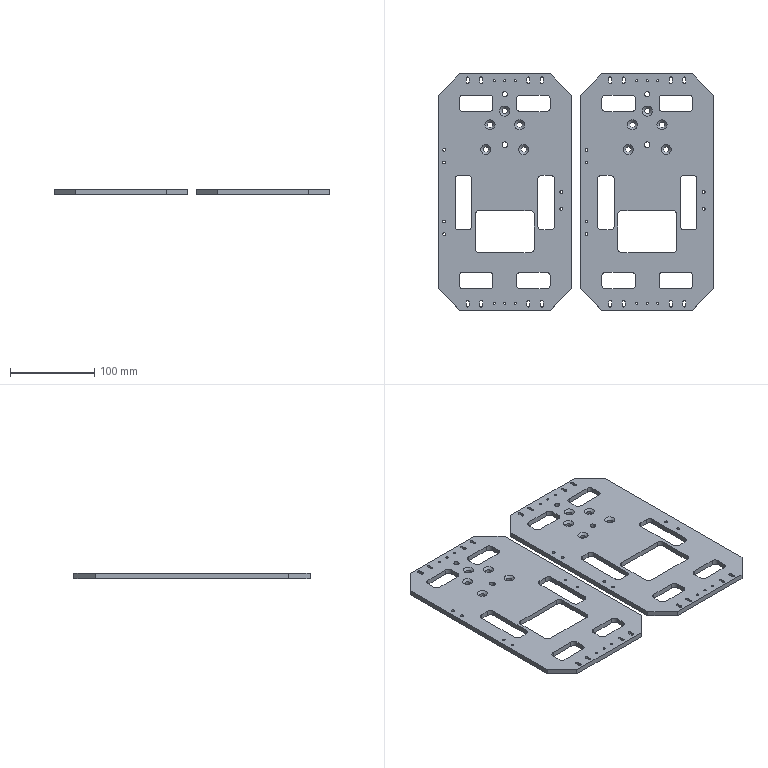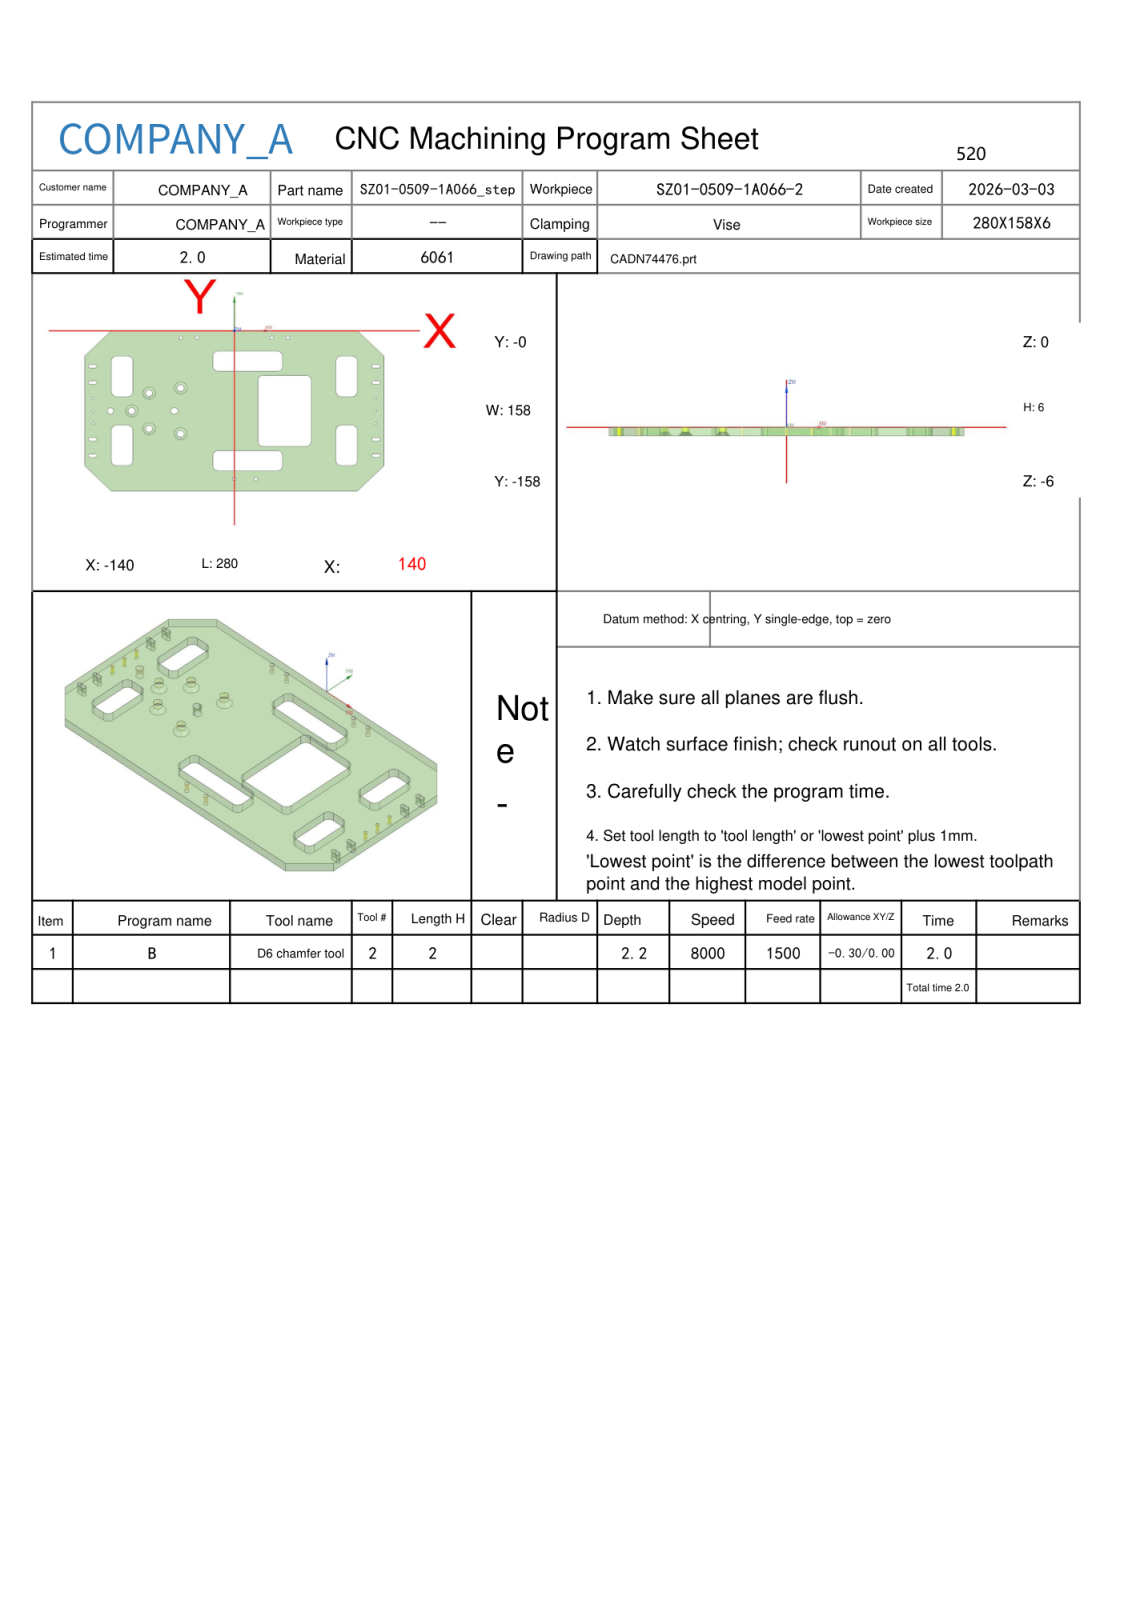NC program | NX | posted by the shop | part box 327 x 280 x 6 mm
Whole program:
%
O0001
(Machine time: 2.11 MIN)
(===Total Tool:1===)
(T2=D6 chamfer tool   D=6.   R=0.   D-  H02 Z=-2.2  )
G80 G90 G17 G49 G40
G91 G28 Z0
M01
N1 T02 M06
(D6 chamfer tool  D=6. R=0. H=02 ce=-0.30 di=0.00)
G00 G90 G54 X114.3 Y-32.86 M03 S7000
G43 H02 Z50.
M08
Z2.5
G01 Y-29.839 Z1.401 F1500.
X114.263 Y-29.412 Z1.245
X114.183 Y-28.99 Z1.088
X114.062 Y-28.579 Z.932
X113.9 Y-28.182 Z.776
X113.699 Y-27.802 Z.62
X113.462 Y-27.445 Z.464
X113.191 Y-27.113 Z.308
X112.887 Y-26.809 Z.151
X112.555 Y-26.538 Z-.005
X112.198 Y-26.301 Z-.161
X111.818 Y-26.1 Z-.317
X111.421 Y-25.938 Z-.473
X111.01 Y-25.817 Z-.629
X110.588 Y-25.737 Z-.785
X110.161 Y-25.7 Z-.942
X110. Z-1.
X100.
G03 X95.7 Y-30. I0.0 J-4.3
G01 Y-60.
G03 X100. Y-64.3 I4.3 J0.0
G01 X110.
G03 X114.3 Y-60. I0.0 J4.3
G01 Y-30.
G03 X110. Y-25.7 I-4.3 J0.0
G01 X109.5
Z1.5
G00 Z50.
X132.93 Y-36.
Z2.5
G01 X134.878 Z1.791
X135.077 Y-35.964 Z1.717
X135.265 Y-35.889 Z1.644
X135.434 Y-35.777 Z1.57
X135.577 Y-35.634 Z1.496
X135.689 Y-35.465 Z1.422
X135.764 Y-35.277 Z1.349
X135.8 Y-35.078 Z1.275
Y-34.922 Z1.219
X135.764 Y-34.723 Z1.145
X135.689 Y-34.535 Z1.071
X135.577 Y-34.366 Z.997
X135.434 Y-34.223 Z.924
X135.265 Y-34.111 Z.85
X135.077 Y-34.036 Z.776
X134.878 Y-34. Z.702
X130.2 Z-1.
G03 X129.2 Y-35. I0.0 J-1.
X130.2 Y-36. I1. J0.0
G01 X134.8
G03 X135.8 Y-35. I0.0 J1.
X134.8 Y-34. I-1. J0.0
G01 X130.2
G03 X129.721 Y-34.122 I0.0 J-1.
G01 Z1.5
G00 Z50.
X132.93 Y-52.
Z2.5
G01 X134.878 Z1.791
X135.077 Y-51.964 Z1.717
X135.265 Y-51.889 Z1.644
X135.434 Y-51.777 Z1.57
X135.577 Y-51.634 Z1.496
X135.689 Y-51.465 Z1.422
X135.764 Y-51.277 Z1.349
X135.8 Y-51.078 Z1.275
Y-50.922 Z1.219
X135.764 Y-50.723 Z1.145
X135.689 Y-50.535 Z1.071
X135.577 Y-50.366 Z.997
X135.434 Y-50.223 Z.924
X135.265 Y-50.111 Z.85
X135.077 Y-50.036 Z.776
X134.878 Y-50. Z.702
X130.2 Z-1.
G03 X129.2 Y-51. I0.0 J-1.
X130.2 Y-52. I1. J0.0
G01 X134.8
G03 X135.8 Y-51. I0.0 J1.
X134.8 Y-50. I-1. J0.0
G01 X130.2
G03 X129.721 Y-50.122 I0.0 J-1.
G01 Z1.5
G00 Z50.
X132.93 Y-108.
Z2.5
G01 X134.878 Z1.791
X135.077 Y-107.964 Z1.717
X135.265 Y-107.889 Z1.644
X135.434 Y-107.777 Z1.57
X135.577 Y-107.634 Z1.496
X135.689 Y-107.465 Z1.422
X135.764 Y-107.277 Z1.349
X135.8 Y-107.078 Z1.275
Y-106.922 Z1.219
X135.764 Y-106.723 Z1.145
X135.689 Y-106.535 Z1.071
X135.577 Y-106.366 Z.997
X135.434 Y-106.223 Z.924
X135.265 Y-106.111 Z.85
X135.077 Y-106.036 Z.776
X134.878 Y-106. Z.702
X130.2 Z-1.
G03 X129.2 Y-107. I0.0 J-1.
X130.2 Y-108. I1. J0.0
G01 X134.8
G03 X135.8 Y-107. I0.0 J1.
X134.8 Y-106. I-1. J0.0
G01 X130.2
G03 X129.721 Y-106.122 I0.0 J-1.
G01 Z1.5
G00 Z50.
X132.93 Y-124.
Z2.5
G01 X134.878 Z1.791
X135.077 Y-123.964 Z1.717
X135.265 Y-123.889 Z1.644
X135.434 Y-123.777 Z1.57
X135.577 Y-123.634 Z1.496
X135.689 Y-123.465 Z1.422
X135.764 Y-123.277 Z1.349
X135.8 Y-123.078 Z1.275
Y-122.922 Z1.219
X135.764 Y-122.723 Z1.145
X135.689 Y-122.535 Z1.071
X135.577 Y-122.366 Z.997
X135.434 Y-122.223 Z.924
X135.265 Y-122.111 Z.85
X135.077 Y-122.036 Z.776
X134.878 Y-122. Z.702
X130.2 Z-1.
G03 X129.2 Y-123. I0.0 J-1.
X130.2 Y-124. I1. J0.0
G01 X134.8
G03 X135.8 Y-123. I0.0 J1.
X134.8 Y-122. I-1. J0.0
G01 X130.2
G03 X129.721 Y-122.122 I0.0 J-1.
G01 Z1.5
G00 Z50.
X114.3 Y-100.86
Z2.5
G01 Y-97.839 Z1.401
X114.263 Y-97.412 Z1.245
X114.183 Y-96.99 Z1.088
X114.062 Y-96.579 Z.932
X113.9 Y-96.182 Z.776
X113.699 Y-95.802 Z.62
X113.462 Y-95.445 Z.464
X113.191 Y-95.113 Z.308
X112.887 Y-94.809 Z.151
X112.555 Y-94.538 Z-.005
X112.198 Y-94.301 Z-.161
X111.818 Y-94.1 Z-.317
X111.421 Y-93.938 Z-.473
X111.01 Y-93.817 Z-.629
X110.588 Y-93.737 Z-.785
X110.161 Y-93.7 Z-.942
X110. Z-1.
X100.
G03 X95.7 Y-98. I0.0 J-4.3
G01 Y-128.
G03 X100. Y-132.3 I4.3 J0.0
G01 X110.
G03 X114.3 Y-128. I0.0 J4.3
G01 Y-98.
G03 X110. Y-93.7 I-4.3 J0.0
G01 X109.5
Z1.5
G00 Z50.
X71.3 Y-51.86
Z2.5
G01 Y-48.839 Z1.401
X71.263 Y-48.412 Z1.245
X71.183 Y-47.99 Z1.088
X71.062 Y-47.579 Z.932
X70.9 Y-47.182 Z.776
X70.699 Y-46.802 Z.62
X70.462 Y-46.445 Z.464
X70.191 Y-46.113 Z.308
X69.887 Y-45.809 Z.151
X69.555 Y-45.538 Z-.005
X69.198 Y-45.301 Z-.161
X68.818 Y-45.1 Z-.317
X68.421 Y-44.938 Z-.473
X68.01 Y-44.817 Z-.629
X67.588 Y-44.737 Z-.785
X67.161 Y-44.7 Z-.942
X67. Z-1.
X27.
G03 X22.7 Y-49. I0.0 J-4.3
G01 Y-109.
G03 X27. Y-113.3 I4.3 J0.0
G01 X67.
G03 X71.3 Y-109. I0.0 J4.3
G01 Y-49.
G03 X67. Y-44.7 I-4.3 J0.0
G01 X66.5
Z1.5
G00 Z50.
X44.3 Y-125.86
Z2.5
G01 Y-122.839 Z1.401
X44.263 Y-122.412 Z1.245
X44.183 Y-121.99 Z1.088
X44.062 Y-121.579 Z.932
X43.9 Y-121.182 Z.776
X43.699 Y-120.802 Z.62
X43.462 Y-120.445 Z.464
X43.191 Y-120.113 Z.308
X42.887 Y-119.809 Z.151
X42.555 Y-119.538 Z-.005
X42.198 Y-119.301 Z-.161
X41.818 Y-119.1 Z-.317
X41.421 Y-118.938 Z-.473
X41.01 Y-118.817 Z-.629
X40.588 Y-118.737 Z-.785
X40.161 Y-118.7 Z-.942
X40. Z-1.
X-15.
G03 X-19.3 Y-123. I0.0 J-4.3
G01 Y-133.
G03 X-15. Y-137.3 I4.3 J0.0
G01 X40.
G03 X44.3 Y-133. I0.0 J4.3
G01 Y-123.
G03 X40. Y-118.7 I-4.3 J0.0
G01 X39.5
Z1.5
G00 Z50.
X140.7 Y-124.046
Z2.5
G01 Y-132.876 Z-.714
Y-132.953 Z-.742
X140.662 Y-133.16 Z-.819
X140.581 Y-133.355 Z-.895
X140.462 Y-133.528 Z-.972
X140.407 Y-133.583 Z-1.
X115.583 Y-158.407
G02 X114.876 Y-158.7 I-.707 J.707
G01 X-114.876
G02 X-115.583 Y-158.407 I0.0 J1.
G01 X-140.407 Y-133.583
G02 X-140.7 Y-132.876 I.707 J.707
G01 Y-25.124
G02 X-140.407 Y-24.417 I1. J0.0
G01 X-115.583 Y.407
G02 X-114.876 Y.7 I.707 J-.707
G01 X114.876
G02 X115.583 Y.407 I0.0 J-1.
G01 X140.407 Y-24.417
G02 X140.7 Y-25.124 I-.707 J-.707
G01 Y-132.876
G02 X140.407 Y-133.583 I-1. J0.0
G01 X140.054 Y-133.936
Z1.5
G00 Z50.
X44.3 Y-27.86
Z2.5
G01 Y-24.839 Z1.401
X44.263 Y-24.412 Z1.245
X44.183 Y-23.99 Z1.088
X44.062 Y-23.579 Z.932
X43.9 Y-23.182 Z.776
X43.699 Y-22.802 Z.62
X43.462 Y-22.445 Z.464
X43.191 Y-22.113 Z.308
X42.887 Y-21.809 Z.151
X42.555 Y-21.538 Z-.005
X42.198 Y-21.301 Z-.161
X41.818 Y-21.1 Z-.317
X41.421 Y-20.938 Z-.473
X41.01 Y-20.817 Z-.629
X40.588 Y-20.737 Z-.785
X40.161 Y-20.7 Z-.942
X40. Z-1.
X-15.
G03 X-19.3 Y-25. I0.0 J-4.3
G01 Y-35.
G03 X-15. Y-39.3 I4.3 J0.0
G01 X40.
G03 X44.3 Y-35. I0.0 J4.3
G01 Y-25.
G03 X40. Y-20.7 I-4.3 J0.0
G01 X39.5
Z1.5
G00 Z50.
X-48.88 Y-54.293
Z2.5
G01 X-49.08 Y-54.175 Z2.416
X-49.399 Y-54.04 Z2.29
X-49.733 Y-53.949 Z2.163
X-50.077 Y-53.903 Z2.037
X-50.423 Z1.911
X-50.767 Y-53.949 Z1.785
X-51.101 Y-54.04 Z1.659
X-51.42 Y-54.175 Z1.533
X-51.719 Y-54.351 Z1.407
X-51.991 Y-54.565 Z1.281
X-52.233 Y-54.813 Z1.154
X-52.439 Y-55.092 Z1.028
X-52.564 Y-55.308 Z.937
X-52.702 Y-55.626 Z.811
X-52.796 Y-55.96 Z.685
X-52.846 Y-56.303 Z.559
X-52.849 Y-56.649 Z.433
X-52.806 Y-56.993 Z.307
X-52.718 Y-57.328 Z.181
X-52.586 Y-57.649 Z.054
X-52.413 Y-57.949 Z-.072
X-52.201 Y-58.223 Z-.198
X-51.955 Y-58.467 Z-.324
X-51.678 Y-58.676 Z-.45
X-51.377 Y-58.846 Z-.576
X-51.055 Y-58.975 Z-.702
X-50.719 Y-59.06 Z-.828
X-50.375 Y-59.1 Z-.955
X-50.25 Z-1.
G03 X-47.65 Y-56.5 I0.0 J2.6
X-50.25 Y-53.9 I-2.6 J0.0
X-52.85 Y-56.5 I0.0 J-2.6
X-50.25 Y-59.1 I2.6 J0.0
X-49.753 Y-59.052 I0.0 J2.6
G01 Z1.5
G00 Z50.
X-56.884 Y-81.268
Z2.5
G01 X-56.618 Y-81.3 Z2.402
X-55.382 Z1.953
X-55.077 Y-81.264 Z1.841
X-54.78 Y-81.187 Z1.729
X-54.495 Y-81.072 Z1.617
X-54.228 Y-80.92 Z1.505
X-53.984 Y-80.733 Z1.393
X-53.767 Y-80.516 Z1.282
X-53.58 Y-80.272 Z1.17
X-53.428 Y-80.005 Z1.058
X-53.313 Y-79.72 Z.946
X-53.236 Y-79.423 Z.834
X-53.2 Y-79.118 Z.722
Y-78.882 Z.637
X-53.236 Y-78.577 Z.525
X-53.313 Y-78.28 Z.413
X-53.428 Y-77.995 Z.301
X-53.58 Y-77.728 Z.19
X-53.767 Y-77.484 Z.078
X-53.984 Y-77.267 Z-.034
X-54.228 Y-77.08 Z-.146
X-54.495 Y-76.928 Z-.258
X-54.78 Y-76.813 Z-.37
X-55.077 Y-76.736 Z-.481
X-55.382 Y-76.7 Z-.593
X-56.5 Z-1.
G03 X-58.8 Y-79. I0.0 J-2.3
X-56.5 Y-81.3 I2.3 J0.0
G01 X-55.5
G03 X-53.2 Y-79. I0.0 J2.3
X-55.5 Y-76.7 I-2.3 J0.0
G01 X-56.5
G03 X-56.996 Y-76.754 I0.0 J-2.3
G01 Z1.5
G00 Z50.
X-48.88 Y-99.293
Z2.5
G01 X-49.08 Y-99.175 Z2.416
X-49.399 Y-99.04 Z2.29
X-49.733 Y-98.949 Z2.163
X-50.077 Y-98.903 Z2.037
X-50.423 Z1.911
X-50.767 Y-98.949 Z1.785
X-51.101 Y-99.04 Z1.659
X-51.42 Y-99.175 Z1.533
X-51.719 Y-99.351 Z1.407
X-51.991 Y-99.565 Z1.281
X-52.233 Y-99.813 Z1.154
X-52.439 Y-100.092 Z1.028
X-52.564 Y-100.308 Z.937
X-52.702 Y-100.626 Z.811
X-52.796 Y-100.96 Z.685
X-52.846 Y-101.303 Z.559
X-52.849 Y-101.649 Z.433
X-52.806 Y-101.993 Z.307
X-52.718 Y-102.328 Z.181
X-52.586 Y-102.649 Z.054
X-52.413 Y-102.949 Z-.072
X-52.201 Y-103.223 Z-.198
X-51.955 Y-103.467 Z-.324
X-51.678 Y-103.676 Z-.45
X-51.377 Y-103.846 Z-.576
X-51.055 Y-103.975 Z-.702
X-50.719 Y-104.06 Z-.828
X-50.375 Y-104.1 Z-.955
X-50.25 Z-1.
G03 X-47.65 Y-101.5 I0.0 J2.6
X-50.25 Y-98.9 I-2.6 J0.0
X-52.85 Y-101.5 I0.0 J-2.6
X-50.25 Y-104.1 I2.6 J0.0
X-49.753 Y-104.052 I0.0 J2.6
G01 Z1.5
G00 Z50.
X-78.38 Y-94.293
Z2.5
G01 X-78.58 Y-94.175 Z2.416
X-78.899 Y-94.04 Z2.29
X-79.233 Y-93.949 Z2.163
X-79.577 Y-93.903 Z2.037
X-79.923 Z1.911
X-80.267 Y-93.949 Z1.785
X-80.601 Y-94.04 Z1.659
X-80.92 Y-94.175 Z1.533
X-81.219 Y-94.351 Z1.407
X-81.491 Y-94.565 Z1.281
X-81.733 Y-94.813 Z1.154
X-81.939 Y-95.092 Z1.028
X-82.064 Y-95.308 Z.937
X-82.202 Y-95.626 Z.811
X-82.296 Y-95.96 Z.685
X-82.346 Y-96.303 Z.559
X-82.349 Y-96.649 Z.433
X-82.306 Y-96.993 Z.307
X-82.218 Y-97.328 Z.181
X-82.086 Y-97.649 Z.054
X-81.913 Y-97.949 Z-.072
X-81.701 Y-98.223 Z-.198
X-81.455 Y-98.467 Z-.324
X-81.178 Y-98.676 Z-.45
X-80.877 Y-98.846 Z-.576
X-80.555 Y-98.975 Z-.702
X-80.219 Y-99.06 Z-.828
X-79.875 Y-99.1 Z-.955
X-79.75 Z-1.
G03 X-77.15 Y-96.5 I0.0 J2.6
X-79.75 Y-93.9 I-2.6 J0.0
X-82.35 Y-96.5 I0.0 J-2.6
X-79.75 Y-99.1 I2.6 J0.0
X-79.253 Y-99.052 I0.0 J2.6
G01 Z1.5
G00 Z50.
X-95.7 Y-100.86
Z2.5
G01 Y-97.839 Z1.401
X-95.737 Y-97.412 Z1.245
X-95.817 Y-96.99 Z1.088
X-95.938 Y-96.579 Z.932
X-96.1 Y-96.182 Z.776
X-96.301 Y-95.802 Z.62
X-96.538 Y-95.445 Z.464
X-96.809 Y-95.113 Z.308
X-97.113 Y-94.809 Z.151
X-97.445 Y-94.538 Z-.005
X-97.802 Y-94.301 Z-.161
X-98.182 Y-94.1 Z-.317
X-98.579 Y-93.938 Z-.473
X-98.99 Y-93.817 Z-.629
X-99.412 Y-93.737 Z-.785
X-99.839 Y-93.7 Z-.942
X-100. Z-1.
X-110.
G03 X-114.3 Y-98. I0.0 J-4.3
G01 Y-128.
G03 X-110. Y-132.3 I4.3 J0.0
G01 X-100.
G03 X-95.7 Y-128. I0.0 J4.3
G01 Y-98.
G03 X-100. Y-93.7 I-4.3 J0.0
G01 X-100.5
Z1.5
G00 Z50.
X-132.07 Y-124.
Z2.5
G01 X-130.122 Z1.791
X-129.923 Y-123.964 Z1.717
X-129.735 Y-123.889 Z1.644
X-129.566 Y-123.777 Z1.57
X-129.423 Y-123.634 Z1.496
X-129.311 Y-123.465 Z1.422
X-129.236 Y-123.277 Z1.349
X-129.2 Y-123.078 Z1.275
Y-122.922 Z1.219
X-129.236 Y-122.723 Z1.145
X-129.311 Y-122.535 Z1.071
X-129.423 Y-122.366 Z.997
X-129.566 Y-122.223 Z.924
X-129.735 Y-122.111 Z.85
X-129.923 Y-122.036 Z.776
X-130.122 Y-122. Z.702
X-134.8 Z-1.
G03 X-135.8 Y-123. I0.0 J-1.
X-134.8 Y-124. I1. J0.0
G01 X-130.2
G03 X-129.2 Y-123. I0.0 J1.
X-130.2 Y-122. I-1. J0.0
G01 X-134.8
G03 X-135.279 Y-122.122 I0.0 J-1.
G01 Z1.5
G00 Z50.
X-132.07 Y-108.
Z2.5
G01 X-130.122 Z1.791
X-129.923 Y-107.964 Z1.717
X-129.735 Y-107.889 Z1.644
X-129.566 Y-107.777 Z1.57
X-129.423 Y-107.634 Z1.496
X-129.311 Y-107.465 Z1.422
X-129.236 Y-107.277 Z1.349
X-129.2 Y-107.078 Z1.275
Y-106.922 Z1.219
X-129.236 Y-106.723 Z1.145
X-129.311 Y-106.535 Z1.071
X-129.423 Y-106.366 Z.997
X-129.566 Y-106.223 Z.924
X-129.735 Y-106.111 Z.85
X-129.923 Y-106.036 Z.776
X-130.122 Y-106. Z.702
X-134.8 Z-1.
G03 X-135.8 Y-107. I0.0 J-1.
X-134.8 Y-108. I1. J0.0
G01 X-130.2
G03 X-129.2 Y-107. I0.0 J1.
X-130.2 Y-106. I-1. J0.0
G01 X-134.8
G03 X-135.279 Y-106.122 I0.0 J-1.
G01 Z1.5
G00 Z50.
X-94.63 Y-76.793
Z2.5
G01 X-94.83 Y-76.675 Z2.416
X-95.149 Y-76.54 Z2.29
X-95.483 Y-76.449 Z2.163
X-95.827 Y-76.403 Z2.037
X-96.173 Z1.911
X-96.517 Y-76.449 Z1.785
X-96.851 Y-76.54 Z1.659
X-97.17 Y-76.675 Z1.533
X-97.469 Y-76.851 Z1.407
X-97.741 Y-77.065 Z1.281
X-97.983 Y-77.313 Z1.154
X-98.189 Y-77.592 Z1.028
X-98.314 Y-77.808 Z.937
X-98.452 Y-78.126 Z.811
X-98.546 Y-78.46 Z.685
X-98.596 Y-78.803 Z.559
X-98.599 Y-79.149 Z.433
X-98.556 Y-79.493 Z.307
X-98.468 Y-79.828 Z.181
X-98.336 Y-80.149 Z.054
X-98.163 Y-80.449 Z-.072
X-97.951 Y-80.723 Z-.198
X-97.705 Y-80.967 Z-.324
X-97.428 Y-81.176 Z-.45
X-97.127 Y-81.346 Z-.576
X-96.805 Y-81.475 Z-.702
X-96.469 Y-81.56 Z-.828
X-96.125 Y-81.6 Z-.955
X-96. Z-1.
G03 X-93.4 Y-79. I0.0 J2.6
X-96. Y-76.4 I-2.6 J0.0
X-98.6 Y-79. I0.0 J-2.6
X-96. Y-81.6 I2.6 J0.0
X-95.503 Y-81.552 I0.0 J2.6
G01 Z1.5
G00 Z50.
X-78.38 Y-59.293
Z2.5
G01 X-78.58 Y-59.175 Z2.416
X-78.899 Y-59.04 Z2.29
X-79.233 Y-58.949 Z2.163
X-79.577 Y-58.903 Z2.037
X-79.923 Z1.911
X-80.267 Y-58.949 Z1.785
X-80.601 Y-59.04 Z1.659
X-80.92 Y-59.175 Z1.533
X-81.219 Y-59.351 Z1.407
X-81.491 Y-59.565 Z1.281
X-81.733 Y-59.813 Z1.154
X-81.939 Y-60.092 Z1.028
X-82.064 Y-60.308 Z.937
X-82.202 Y-60.626 Z.811
X-82.296 Y-60.96 Z.685
X-82.346 Y-61.303 Z.559
X-82.349 Y-61.649 Z.433
X-82.306 Y-61.993 Z.307
X-82.218 Y-62.328 Z.181
X-82.086 Y-62.649 Z.054
X-81.913 Y-62.949 Z-.072
X-81.701 Y-63.223 Z-.198
X-81.455 Y-63.467 Z-.324
X-81.178 Y-63.676 Z-.45
X-80.877 Y-63.846 Z-.576
X-80.555 Y-63.975 Z-.702
X-80.219 Y-64.06 Z-.828
X-79.875 Y-64.1 Z-.955
X-79.75 Z-1.
G03 X-77.15 Y-61.5 I0.0 J2.6
X-79.75 Y-58.9 I-2.6 J0.0
X-82.35 Y-61.5 I0.0 J-2.6
X-79.75 Y-64.1 I2.6 J0.0
X-79.253 Y-64.052 I0.0 J2.6
G01 Z1.5
G00 Z50.
X-95.7 Y-32.86
Z2.5
G01 Y-29.839 Z1.401
X-95.737 Y-29.412 Z1.245
X-95.817 Y-28.99 Z1.088
X-95.938 Y-28.579 Z.932
X-96.1 Y-28.182 Z.776
X-96.301 Y-27.802 Z.62
X-96.538 Y-27.445 Z.464
X-96.809 Y-27.113 Z.308
X-97.113 Y-26.809 Z.151
X-97.445 Y-26.538 Z-.005
X-97.802 Y-26.301 Z-.161
X-98.182 Y-26.1 Z-.317
X-98.579 Y-25.938 Z-.473
X-98.99 Y-25.817 Z-.629
X-99.412 Y-25.737 Z-.785
X-99.839 Y-25.7 Z-.942
X-100. Z-1.
X-110.
G03 X-114.3 Y-30. I0.0 J-4.3
G01 Y-60.
G03 X-110. Y-64.3 I4.3 J0.0
G01 X-100.
G03 X-95.7 Y-60. I0.0 J4.3
G01 Y-30.
G03 X-100. Y-25.7 I-4.3 J0.0
G01 X-100.5
Z1.5
G00 Z50.
X-132.07 Y-52.
Z2.5
G01 X-130.122 Z1.791
X-129.923 Y-51.964 Z1.717
X-129.735 Y-51.889 Z1.644
X-129.566 Y-51.777 Z1.57
X-129.423 Y-51.634 Z1.496
X-129.311 Y-51.465 Z1.422
X-129.236 Y-51.277 Z1.349
X-129.2 Y-51.078 Z1.275
Y-50.922 Z1.219
X-129.236 Y-50.723 Z1.145
X-129.311 Y-50.535 Z1.071
X-129.423 Y-50.366 Z.997
X-129.566 Y-50.223 Z.924
X-129.735 Y-50.111 Z.85
X-129.923 Y-50.036 Z.776
X-130.122 Y-50. Z.702
X-134.8 Z-1.
G03 X-135.8 Y-51. I0.0 J-1.
X-134.8 Y-52. I1. J0.0
G01 X-130.2
G03 X-129.2 Y-51. I0.0 J1.
X-130.2 Y-50. I-1. J0.0
G01 X-134.8
G03 X-135.279 Y-50.122 I0.0 J-1.
G01 Z1.5
G00 Z50.
X-132.07 Y-36.
Z2.5
G01 X-130.122 Z1.791
X-129.923 Y-35.964 Z1.717
X-129.735 Y-35.889 Z1.644
X-129.566 Y-35.777 Z1.57
X-129.423 Y-35.634 Z1.496
X-129.311 Y-35.465 Z1.422
X-129.236 Y-35.277 Z1.349
X-129.2 Y-35.078 Z1.275
Y-34.922 Z1.219
X-129.236 Y-34.723 Z1.145
X-129.311 Y-34.535 Z1.071
X-129.423 Y-34.366 Z.997
X-129.566 Y-34.223 Z.924
X-129.735 Y-34.111 Z.85
X-129.923 Y-34.036 Z.776
X-130.122 Y-34. Z.702
X-134.8 Z-1.
G03 X-135.8 Y-35. I0.0 J-1.
X-134.8 Y-36. I1. J0.0
G01 X-130.2
G03 X-129.2 Y-35. I0.0 J1.
X-130.2 Y-34. I-1. J0.0
G01 X-134.8
G03 X-135.279 Y-34.122 I0.0 J-1.
G01 Z1.5
G00 Z50.
G00 G90 X-132. Y-91.5 M03 S8000
Z50.
G98 G81 X-132. Y-91.5 Z-1.75 R3. F1000.
Y-79.
Y-66.5
X132.
Y-79.
Y-91.5
G80
G00 Z50.
G00 G90 X20. Y-146. M03 S8000
Z50.
G98 G81 X20. Y-146. Z-2.2 R3. F1000.
X0.0
G80
G00 Z50.
G00 G90 X50. Y-7. M03 S8000
Z50.
G98 G81 X50. Y-7. Z-2. R3. F1000.
X35.
X-35.
X-50.
G80
G00 Z50.
G00 G90 X-117.981 Y-80.17 M03 S7000
Z50.
Z2.5
G01 X-117.933 Y-80.252 Z2.465 F1500.
X-117.736 Y-80.513 Z2.346
X-117.504 Y-80.744 Z2.227
X-117.241 Y-80.94 Z2.108
X-116.954 Y-81.096 Z1.989
X-116.647 Y-81.21 Z1.87
X-116.327 Y-81.28 Z1.75
X-116. Y-81.303 Z1.631
X-115.673 Y-81.28 Z1.512
X-115.353 Y-81.21 Z1.393
X-115.046 Y-81.096 Z1.274
X-114.759 Y-80.94 Z1.154
X-114.496 Y-80.744 Z1.035
X-114.264 Y-80.513 Z.916
X-114.067 Y-80.252 Z.797
X-113.949 Y-80.048 Z.711
X-113.821 Y-79.747 Z.592
X-113.738 Y-79.43 Z.473
X-113.699 Y-79.105 Z.354
X-113.708 Y-78.778 Z.235
X-113.762 Y-78.455 Z.115
X-113.862 Y-78.143 Z-.004
X-114.006 Y-77.849 Z-.123
X-114.189 Y-77.577 Z-.242
X-114.409 Y-77.335 Z-.361
X-114.661 Y-77.126 Z-.48
X-114.941 Y-76.955 Z-.6
X-115.241 Y-76.826 Z-.719
X-115.557 Y-76.74 Z-.838
X-115.882 Y-76.7 Z-.957
X-116. Z-1.
G03 X-118.3 Y-79. I0.0 J-2.3
X-116. Y-81.3 I2.3 J0.0
X-113.7 Y-79. I0.0 J2.3
X-116. Y-76.7 I-2.3 J0.0
X-116.496 Y-76.754 I0.0 J-2.3
G01 Z1.5
G00 Z50.
M05
M09
G91 G28 Z0.0
G91 G28 Y0.0
M30
%